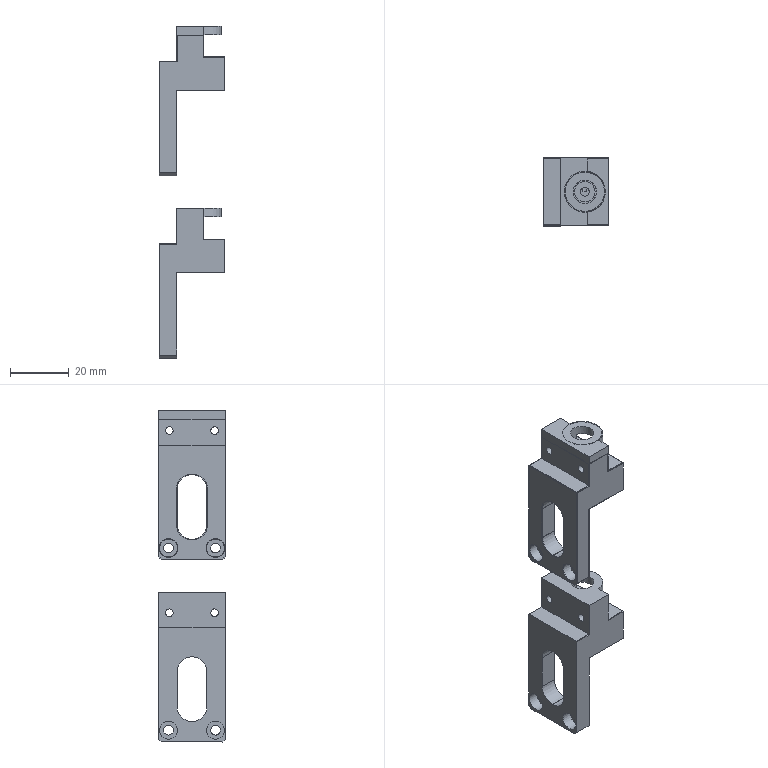CAM job | NX | 3+2 milling, drilling | part box 22.4 x 23 x 113 mm | stock box 25 x 25 x 118 mm
Tools:
number,name,description,diameter,corner_radius,flute_length,length,flutes
4,D4,平底铣刀-粗,4.0,0.0,25.0,75.0,2
6,D6,平底铣刀-粗,6.0,0.0,25.0,75.0,2
9,D10,平底铣刀-粗,10.0,0.0,35.0,75.0,2
11,D4-J,平底铣刀-精,4.0,0.0,50.0,75.0,2
7,D6-J,平底铣刀-精,6.0,0.0,25.0,75.0,2
10,D10-J,平底铣刀-精,10.0,0.0,35.0,75.0,2
1,D80R0.8飞刀,圆鼻刀-粗,80.0,0.8,50.0,75.0,2
1,D80R0.8飞刀-J,圆鼻刀-精,80.0,0.8,50.0,75.0,2
2,D6倒角刀,倒角刀,6.0,0.0,3.0,25.0,2
20,M3X0.5,丝锥,2.5,0.0,35.0,50.0,2
12,ZT2.6,钻头,2.6,0.0,35.0,50.0,2
17,ZT3,钻头,3.0,0.0,35.0,50.0,2
13,钻头3.3,Twist Drill 3.3 mm,3.3,0.0,35.0,35.008,2
Operations:
program,operation,operation_type,tool,method,geometry_group,spindle_rpm,surface_speed,feed_per_tooth,feed_cut,feed_plunge,cut_length_mm,path_length_mm,cut_time_min,machine_time_min
C,等高螺旋开粗-中_COPY_1,ZLevelMilling,D10,分层开粗-切深K-步距G,W-C,8000.0,251.327,0.125,2000.0,100.0,639.714,680.614,0.3199,0.3239
C,通用打点-深0.8,Operation,D6倒角刀,NONE,W-C,8000.0,150.796,0.0312,500.0,90.0,1.8,43.6,0.0036,0.0078
C,三段孔-G83钻孔,Operation,ZT3,NONE,W-C,1500.0,14.137,0.04,120.0,90.0,20.5,81.0,0.1708,0.1769
C,三段孔-铣孔开粗1_1,CylinderMilling,D4,NONE,W-C,8000.0,100.531,0.075,1200.0,100.0,508.614,559.614,0.4238,0.4289
C,三段孔-铣孔开粗2_1,CylinderMilling,D4,NONE,W-C,8000.0,100.531,0.075,1200.0,100.0,80.513,144.713,0.0671,0.0735
C,铣倒角_2,PlanarMilling,D6倒角刀,METHOD,W-C,8000.0,150.796,0.05,800.0,100.0,31.706,73.106,0.0396,0.0438
C,平面去毛刺6X45L_COPY_1,SurfaceContour,D6倒角刀,爬面_倒角-切深0-步距G,W-C,6500.0,122.519,0.1154,1500.0,100.0,128.315,210.372,0.0855,0.0937
C,三段孔-铣孔精光2_1,CylinderMilling,D4-J,精光步距切深关,W-C,8000.0,100.531,0.0312,500.0,100.0,18.757,82.957,0.0375,0.0439
C,底壁铣精光侧面-中_COPY,VolumeBased25DMillingOperation,D4-J,侧刃精光-切深K-步距G,W-C,8000.0,100.531,0.0312,500.0,100.0,56.203,96.705,0.1124,0.1165
C,等高精光-中_COPY_1,ZLevelMilling,D10-J,侧刃精光-切深K-步距G,W-C,8000.0,251.32,0.0625,1000.0,100.0,82.344,96.344,0.0823,0.0837
B,底壁铣飞面一刀开粗_COPY,VolumeBased25DMillingOperation,D80R0.8飞刀,分层开粗-切深K-步距G,W-B,2800.0,703.696,0.5357,3000.0,100.0,1327.164,2516.186,0.4424,0.5613
B,底壁铣飞面一刀精光_COPY,VolumeBased25DMillingOperation,D80R0.8飞刀-J,侧刃精光-切深K-步距G,W-B,4000.0,1005.28,0.125,1000.0,100.0,220.998,256.998,0.221,0.2246
B,底壁铣分层开粗-中_COPY,VolumeBased25DMillingOperation,D10,分层开粗-切深K-步距G,W-B,8000.0,251.32,0.25,4000.0,100.0,14083.271,14284.056,3.521,3.541
B,底壁铣分层开粗-中_COPY_1,VolumeBased25DMillingOperation,D6,分层开粗-切深K-步距G,W-B,8000.0,150.792,0.1875,3000.0,100.0,3344.682,3465.236,1.115,1.127
B,钻倒角_3,Operation,D6倒角刀,METHOD,W-B,8000.0,150.796,0.0625,1000.0,0.0,18.8,194.291,0.0188,0.0363
B,钻倒角_4,Operation,D6倒角刀,METHOD,W-B,8000.0,150.796,0.0625,1000.0,0.0,20.8,218.03,0.0208,0.0405
B,平面去毛刺6X45L_COPY,SurfaceContour,D6倒角刀,爬面_倒角-切深0-步距G,W-B,6500.0,122.519,0.1154,1500.0,100.0,468.157,1236.637,0.3121,0.389
B,底壁铣精光底面-中_COPY,VolumeBased25DMillingOperation,D10-J,精光步距切深关,W-B,8000.0,251.32,0.0625,1000.0,100.0,343.413,503.642,0.3434,0.3594
B,底壁铣精光侧面-中-选底面_COPY,VolumeBased25DMillingOperation,D10-J,侧刃精光-切深K-步距G,W-B,8000.0,251.32,0.0625,1000.0,100.0,100.812,368.209,0.1008,0.1276
B,底壁铣精光底面-中_COPY_1,VolumeBased25DMillingOperation,D6-J,精光步距切深关,W-B,8000.0,150.792,0.0625,1000.0,100.0,177.85,277.55,0.1778,0.1878
B,底壁铣精光侧面-中-选底面_COPY_1,VolumeBased25DMillingOperation,D6-J,侧刃精光-切深K-步距G,W-B,8000.0,150.792,0.0625,1000.0,100.0,159.262,328.821,0.1593,0.1762
A,顶面,FaceMilling,D80R0.8飞刀,侧刃精光-切深K-步距G,W-A,4000.0,1005.31,0.125,1000.0,100.0,207.0,243.0,0.207,0.2106
A,外形粗_2,VolumeBased25DMillingOperation,D10,METHOD,W-A,8000.0,251.327,0.3125,5000.0,80.0,10735.461,10919.761,2.147,2.166
A,底壁粗_1,VolumeBased25DMillingOperation,D6,METHOD,W-A,6000.0,113.0,0.2083,3500.0,100.0,2695.2,3102.004,0.7701,0.8107
A,等高螺旋开粗-中_COPY,ZLevelMilling,D6,分层开粗-切深K-步距G,W-A,8000.0,150.792,0.1875,3000.0,100.0,1096.21,1249.924,0.3654,0.3808
A,打点-深0.8,Operation,D6倒角刀,NONE,W-A,8000.0,150.796,0.0312,500.0,90.0,14.4,248.38,0.0288,0.0522
A,通孔-2-3,Operation,ZT2.6,NONE,W-A,3000.0,24.504,0.0133,80.0,90.0,68.0,283.811,0.85,0.8716
A,沉头孔-钻孔0段,Operation,钻头3.3,NONE,W-A,2800.0,29.028,0.0179,100.0,90.0,39.966,217.002,0.3997,0.4174
A,铣孔开粗D4_1,CylinderMilling,D4,NONE,W-A,8000.0,100.531,0.075,1200.0,100.0,354.564,620.564,0.2955,0.3221
A,铣孔精光D4_1,CylinderMilling,D4,精光步距切深关,W-A,8000.0,100.531,0.0312,500.0,100.0,65.671,331.671,0.1313,0.1579
A,底精_1,VolumeBased25DMillingOperation,D6-J,METHOD,W-A,6000.0,113.0,0.2083,1200.0,100.0,264.6,419.3,0.2205,0.236
A,仅选体,SurfaceContour,D6倒角刀,METHOD,W-A,8000.0,150.796,0.1875,3000.0,100.0,523.599,948.333,0.1745,0.217
A,钻倒角_1,Operation,D6倒角刀,METHOD,W-A,8000.0,150.796,0.0312,500.0,0.0,18.4,191.191,0.0368,0.0541
A,钻倒角_2,Operation,D6倒角刀,METHOD,W-A,8000.0,150.796,0.0312,500.0,0.0,19.2,192.791,0.0384,0.0558
A,铣倒角_1,PlanarMilling,D6倒角刀,NONE,W-A,8000.0,150.796,0.0312,500.0,100.0,111.995,354.511,0.224,0.2482
A,通孔-攻牙M3,Operation,M3X0.5,METHOD,W-A,800.0,6.283,0.0003,0.5,90.0,53.0,253.811,106.0,106.02
A,等高精光-中_COPY,ZLevelMilling,D6-J,侧刃精光-切深K-步距G,W-A,8000.0,150.792,0.0625,1000.0,100.0,85.342,193.946,0.0853,0.0962
A,底侧精_3,VolumeBased25DMillingOperation,D6-J,METHOD,W-A,6000.0,113.0,0.2083,1200.0,100.0,67.873,239.255,0.0566,0.0737
A,外形半精_2,VolumeBased25DMillingOperation,D10-J,METHOD,W-A,8000.0,251.327,0.0625,1000.0,100.0,741.583,1060.197,0.7416,0.7734